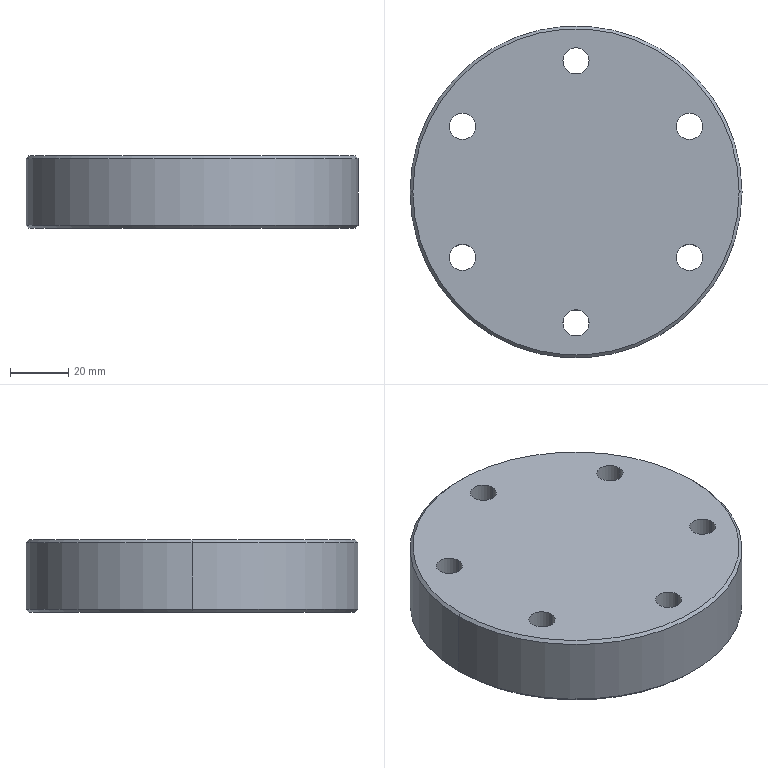Part | SolidWorks | features Chamfer 1, CirPattern 1, Extrusion 1, HoleWzd 1 | 1 solid | 38 faces | box 114 x 114 x 25 mm | volume 237134 mm3 | cylinder 26 | plane 8 | cone 4 | commonest cylinder face diameters 9 x12 15 x12 114 x2
STEP:
#1=CARTESIAN_POINT('',(46.471,22.5,12.));
#2=VERTEX_POINT('',#1);
#3=CARTESIAN_POINT('',(31.471,22.5,12.));
#4=VERTEX_POINT('',#3);
#5=CARTESIAN_POINT('',(38.971,22.5,12.));
#6=DIRECTION('',(0.,0.,-1.));
#7=DIRECTION('',(-1.,0.,0.));
#8=AXIS2_PLACEMENT_3D('',#5,#6,#7);
#9=CIRCLE('',#8,7.5);
#10=EDGE_CURVE('',#2,#4,#9,.T.);
#11=ORIENTED_EDGE('',*,*,#10,.F.);
#12=CARTESIAN_POINT('',(46.471,22.5,0.));
#13=VERTEX_POINT('',#12);
#14=CARTESIAN_POINT('',(46.471,22.5,0.));
#15=DIRECTION('',(0.,0.,-1.));
#16=VECTOR('',#15,1000.);
#17=LINE('',#14,#16);
#18=EDGE_CURVE('',#2,#13,#17,.T.);
#19=ORIENTED_EDGE('',*,*,#18,.T.);
#20=CARTESIAN_POINT('',(31.471,22.5,0.));
#21=VERTEX_POINT('',#20);
#22=CARTESIAN_POINT('',(38.971,22.5,0.));
#23=DIRECTION('',(0.,0.,-1.));
#24=DIRECTION('',(-1.,0.,0.));
#25=AXIS2_PLACEMENT_3D('',#22,#23,#24);
#26=CIRCLE('',#25,7.5);
#27=EDGE_CURVE('',#13,#21,#26,.T.);
#28=ORIENTED_EDGE('',*,*,#27,.T.);
#29=CARTESIAN_POINT('',(31.471,22.5,0.));
#30=DIRECTION('',(0.,0.,-1.));
#31=VECTOR('',#30,1000.);
#32=LINE('',#29,#31);
#33=EDGE_CURVE('',#4,#21,#32,.T.);
#34=ORIENTED_EDGE('',*,*,#33,.F.);
#35=EDGE_LOOP('',(#11,#19,#28,#34));
#36=FACE_OUTER_BOUND('',#35,.T.);
#37=CARTESIAN_POINT('',(38.971,22.5,0.));
#38=DIRECTION('',(0.,0.,-1.));
#39=DIRECTION('',(-1.,0.,0.));
#40=AXIS2_PLACEMENT_3D('',#37,#38,#39);
#41=CYLINDRICAL_SURFACE('',#40,7.5);
#42=ADVANCED_FACE('',(#36),#41,.F.);
#43=CARTESIAN_POINT('',(43.471,22.5,25.));
#44=VERTEX_POINT('',#43);
#45=CARTESIAN_POINT('',(34.471,22.5,25.));
#46=VERTEX_POINT('',#45);
#47=CARTESIAN_POINT('',(38.971,22.5,25.));
#48=DIRECTION('',(0.,0.,-1.));
#49=DIRECTION('',(-1.,0.,0.));
#50=AXIS2_PLACEMENT_3D('',#47,#48,#49);
#51=CIRCLE('',#50,4.5);
#52=EDGE_CURVE('',#44,#46,#51,.T.);
#53=ORIENTED_EDGE('',*,*,#52,.F.);
#54=CARTESIAN_POINT('',(43.471,22.5,12.));
#55=VERTEX_POINT('',#54);
#56=CARTESIAN_POINT('',(43.471,22.5,0.));
#57=DIRECTION('',(0.,0.,-1.));
#58=VECTOR('',#57,1000.);
#59=LINE('',#56,#58);
#60=EDGE_CURVE('',#44,#55,#59,.T.);
#61=ORIENTED_EDGE('',*,*,#60,.T.);
#62=CARTESIAN_POINT('',(34.471,22.5,12.));
#63=VERTEX_POINT('',#62);
#64=CARTESIAN_POINT('',(38.971,22.5,12.));
#65=DIRECTION('',(0.,0.,-1.));
#66=DIRECTION('',(-1.,0.,0.));
#67=AXIS2_PLACEMENT_3D('',#64,#65,#66);
#68=CIRCLE('',#67,4.5);
#69=EDGE_CURVE('',#55,#63,#68,.T.);
#70=ORIENTED_EDGE('',*,*,#69,.T.);
#71=CARTESIAN_POINT('',(34.471,22.5,0.));
#72=DIRECTION('',(0.,0.,-1.));
#73=VECTOR('',#72,1000.);
#74=LINE('',#71,#73);
#75=EDGE_CURVE('',#46,#63,#74,.T.);
#76=ORIENTED_EDGE('',*,*,#75,.F.);
#77=EDGE_LOOP('',(#53,#61,#70,#76));
#78=FACE_OUTER_BOUND('',#77,.T.);
#79=CARTESIAN_POINT('',(38.971,22.5,0.));
#80=DIRECTION('',(0.,0.,-1.));
#81=DIRECTION('',(-1.,0.,0.));
#82=AXIS2_PLACEMENT_3D('',#79,#80,#81);
#83=CYLINDRICAL_SURFACE('',#82,4.5);
#84=ADVANCED_FACE('',(#78),#83,.F.);
#85=CARTESIAN_POINT('',(46.471,-22.5,12.));
#86=VERTEX_POINT('',#85);
#87=CARTESIAN_POINT('',(31.471,-22.5,12.));
#88=VERTEX_POINT('',#87);
#89=CARTESIAN_POINT('',(38.971,-22.5,12.));
#90=DIRECTION('',(0.,0.,-1.));
#91=DIRECTION('',(-1.,0.,0.));
#92=AXIS2_PLACEMENT_3D('',#89,#90,#91);
#93=CIRCLE('',#92,7.5);
#94=EDGE_CURVE('',#86,#88,#93,.T.);
#95=ORIENTED_EDGE('',*,*,#94,.F.);
#96=CARTESIAN_POINT('',(46.471,-22.5,0.));
#97=VERTEX_POINT('',#96);
#98=CARTESIAN_POINT('',(46.471,-22.5,0.));
#99=DIRECTION('',(0.,0.,-1.));
#100=VECTOR('',#99,1000.);
#101=LINE('',#98,#100);
#102=EDGE_CURVE('',#86,#97,#101,.T.);
#103=ORIENTED_EDGE('',*,*,#102,.T.);
#104=CARTESIAN_POINT('',(31.471,-22.5,0.));
#105=VERTEX_POINT('',#104);
#106=CARTESIAN_POINT('',(38.971,-22.5,0.));
#107=DIRECTION('',(0.,0.,-1.));
#108=DIRECTION('',(-1.,0.,0.));
#109=AXIS2_PLACEMENT_3D('',#106,#107,#108);
#110=CIRCLE('',#109,7.5);
#111=EDGE_CURVE('',#97,#105,#110,.T.);
#112=ORIENTED_EDGE('',*,*,#111,.T.);
#113=CARTESIAN_POINT('',(31.471,-22.5,0.));
#114=DIRECTION('',(0.,0.,-1.));
#115=VECTOR('',#114,1000.);
#116=LINE('',#113,#115);
#117=EDGE_CURVE('',#88,#105,#116,.T.);
#118=ORIENTED_EDGE('',*,*,#117,.F.);
#119=EDGE_LOOP('',(#95,#103,#112,#118));
#120=FACE_OUTER_BOUND('',#119,.T.);
#121=CARTESIAN_POINT('',(38.971,-22.5,0.));
#122=DIRECTION('',(0.,0.,-1.));
#123=DIRECTION('',(-1.,0.,0.));
#124=AXIS2_PLACEMENT_3D('',#121,#122,#123);
#125=CYLINDRICAL_SURFACE('',#124,7.5);
#126=ADVANCED_FACE('',(#120),#125,.F.);
#127=CARTESIAN_POINT('',(43.471,-22.5,25.));
#128=VERTEX_POINT('',#127);
#129=CARTESIAN_POINT('',(34.471,-22.5,25.));
#130=VERTEX_POINT('',#129);
#131=CARTESIAN_POINT('',(38.971,-22.5,25.));
#132=DIRECTION('',(0.,0.,-1.));
#133=DIRECTION('',(-1.,0.,0.));
#134=AXIS2_PLACEMENT_3D('',#131,#132,#133);
#135=CIRCLE('',#134,4.5);
#136=EDGE_CURVE('',#128,#130,#135,.T.);
#137=ORIENTED_EDGE('',*,*,#136,.F.);
#138=CARTESIAN_POINT('',(43.471,-22.5,12.));
#139=VERTEX_POINT('',#138);
#140=CARTESIAN_POINT('',(43.471,-22.5,0.));
#141=DIRECTION('',(0.,0.,-1.));
#142=VECTOR('',#141,1000.);
#143=LINE('',#140,#142);
#144=EDGE_CURVE('',#128,#139,#143,.T.);
#145=ORIENTED_EDGE('',*,*,#144,.T.);
#146=CARTESIAN_POINT('',(34.471,-22.5,12.));
#147=VERTEX_POINT('',#146);
#148=CARTESIAN_POINT('',(38.971,-22.5,12.));
#149=DIRECTION('',(0.,0.,-1.));
#150=DIRECTION('',(-1.,0.,0.));
#151=AXIS2_PLACEMENT_3D('',#148,#149,#150);
#152=CIRCLE('',#151,4.5);
#153=EDGE_CURVE('',#139,#147,#152,.T.);
#154=ORIENTED_EDGE('',*,*,#153,.T.);
#155=CARTESIAN_POINT('',(34.471,-22.5,0.));
#156=DIRECTION('',(0.,0.,-1.));
#157=VECTOR('',#156,1000.);
#158=LINE('',#155,#157);
#159=EDGE_CURVE('',#130,#147,#158,.T.);
#160=ORIENTED_EDGE('',*,*,#159,.F.);
#161=EDGE_LOOP('',(#137,#145,#154,#160));
#162=FACE_OUTER_BOUND('',#161,.T.);
#163=CARTESIAN_POINT('',(38.971,-22.5,0.));
#164=DIRECTION('',(0.,0.,-1.));
#165=DIRECTION('',(-1.,0.,0.));
#166=AXIS2_PLACEMENT_3D('',#163,#164,#165);
#167=CYLINDRICAL_SURFACE('',#166,4.5);
#168=ADVANCED_FACE('',(#162),#167,.F.);
#169=CARTESIAN_POINT('',(7.5,-45.,12.));
#170=VERTEX_POINT('',#169);
#171=CARTESIAN_POINT('',(-7.5,-45.,12.));
#172=VERTEX_POINT('',#171);
#173=CARTESIAN_POINT('',(0.,-45.,12.));
#174=DIRECTION('',(0.,0.,-1.));
#175=DIRECTION('',(-1.,0.,0.));
#176=AXIS2_PLACEMENT_3D('',#173,#174,#175);
#177=CIRCLE('',#176,7.5);
#178=EDGE_CURVE('',#170,#172,#177,.T.);
#179=ORIENTED_EDGE('',*,*,#178,.F.);
#180=CARTESIAN_POINT('',(7.5,-45.,0.));
#181=VERTEX_POINT('',#180);
#182=CARTESIAN_POINT('',(7.5,-45.,0.));
#183=DIRECTION('',(0.,0.,-1.));
#184=VECTOR('',#183,1000.);
#185=LINE('',#182,#184);
#186=EDGE_CURVE('',#170,#181,#185,.T.);
#187=ORIENTED_EDGE('',*,*,#186,.T.);
#188=CARTESIAN_POINT('',(-7.5,-45.,0.));
#189=VERTEX_POINT('',#188);
#190=CARTESIAN_POINT('',(0.,-45.,0.));
#191=DIRECTION('',(0.,0.,-1.));
#192=DIRECTION('',(-1.,0.,0.));
#193=AXIS2_PLACEMENT_3D('',#190,#191,#192);
#194=CIRCLE('',#193,7.5);
#195=EDGE_CURVE('',#181,#189,#194,.T.);
#196=ORIENTED_EDGE('',*,*,#195,.T.);
#197=CARTESIAN_POINT('',(-7.5,-45.,0.));
#198=DIRECTION('',(0.,0.,-1.));
#199=VECTOR('',#198,1000.);
#200=LINE('',#197,#199);
#201=EDGE_CURVE('',#172,#189,#200,.T.);
#202=ORIENTED_EDGE('',*,*,#201,.F.);
#203=EDGE_LOOP('',(#179,#187,#196,#202));
#204=FACE_OUTER_BOUND('',#203,.T.);
#205=CARTESIAN_POINT('',(0.,-45.,0.));
#206=DIRECTION('',(0.,0.,-1.));
#207=DIRECTION('',(-1.,0.,0.));
#208=AXIS2_PLACEMENT_3D('',#205,#206,#207);
#209=CYLINDRICAL_SURFACE('',#208,7.5);
#210=ADVANCED_FACE('',(#204),#209,.F.);
#211=CARTESIAN_POINT('',(4.5,-45.,25.));
#212=VERTEX_POINT('',#211);
#213=CARTESIAN_POINT('',(-4.5,-45.,25.));
#214=VERTEX_POINT('',#213);
#215=CARTESIAN_POINT('',(0.,-45.,25.));
#216=DIRECTION('',(0.,0.,-1.));
#217=DIRECTION('',(-1.,0.,0.));
#218=AXIS2_PLACEMENT_3D('',#215,#216,#217);
#219=CIRCLE('',#218,4.5);
#220=EDGE_CURVE('',#212,#214,#219,.T.);
#221=ORIENTED_EDGE('',*,*,#220,.F.);
#222=CARTESIAN_POINT('',(4.5,-45.,12.));
#223=VERTEX_POINT('',#222);
#224=CARTESIAN_POINT('',(4.5,-45.,0.));
#225=DIRECTION('',(0.,0.,-1.));
#226=VECTOR('',#225,1000.);
#227=LINE('',#224,#226);
#228=EDGE_CURVE('',#212,#223,#227,.T.);
#229=ORIENTED_EDGE('',*,*,#228,.T.);
#230=CARTESIAN_POINT('',(-4.5,-45.,12.));
#231=VERTEX_POINT('',#230);
#232=CARTESIAN_POINT('',(0.,-45.,12.));
#233=DIRECTION('',(0.,0.,-1.));
#234=DIRECTION('',(-1.,0.,0.));
#235=AXIS2_PLACEMENT_3D('',#232,#233,#234);
#236=CIRCLE('',#235,4.5);
#237=EDGE_CURVE('',#223,#231,#236,.T.);
#238=ORIENTED_EDGE('',*,*,#237,.T.);
#239=CARTESIAN_POINT('',(-4.5,-45.,0.));
#240=DIRECTION('',(0.,0.,-1.));
#241=VECTOR('',#240,1000.);
#242=LINE('',#239,#241);
#243=EDGE_CURVE('',#214,#231,#242,.T.);
#244=ORIENTED_EDGE('',*,*,#243,.F.);
#245=EDGE_LOOP('',(#221,#229,#238,#244));
#246=FACE_OUTER_BOUND('',#245,.T.);
#247=CARTESIAN_POINT('',(0.,-45.,0.));
#248=DIRECTION('',(0.,0.,-1.));
#249=DIRECTION('',(-1.,0.,0.));
#250=AXIS2_PLACEMENT_3D('',#247,#248,#249);
#251=CYLINDRICAL_SURFACE('',#250,4.5);
#252=ADVANCED_FACE('',(#246),#251,.F.);
#253=CARTESIAN_POINT('',(-31.471,-22.5,12.));
#254=VERTEX_POINT('',#253);
#255=CARTESIAN_POINT('',(-46.471,-22.5,12.));
#256=VERTEX_POINT('',#255);
#257=CARTESIAN_POINT('',(-38.971,-22.5,12.));
#258=DIRECTION('',(0.,0.,-1.));
#259=DIRECTION('',(-1.,0.,0.));
#260=AXIS2_PLACEMENT_3D('',#257,#258,#259);
#261=CIRCLE('',#260,7.5);
#262=EDGE_CURVE('',#254,#256,#261,.T.);
#263=ORIENTED_EDGE('',*,*,#262,.F.);
#264=CARTESIAN_POINT('',(-31.471,-22.5,0.));
#265=VERTEX_POINT('',#264);
#266=CARTESIAN_POINT('',(-31.471,-22.5,0.));
#267=DIRECTION('',(0.,0.,-1.));
#268=VECTOR('',#267,1000.);
#269=LINE('',#266,#268);
#270=EDGE_CURVE('',#254,#265,#269,.T.);
#271=ORIENTED_EDGE('',*,*,#270,.T.);
#272=CARTESIAN_POINT('',(-46.471,-22.5,0.));
#273=VERTEX_POINT('',#272);
#274=CARTESIAN_POINT('',(-38.971,-22.5,0.));
#275=DIRECTION('',(0.,0.,-1.));
#276=DIRECTION('',(-1.,0.,0.));
#277=AXIS2_PLACEMENT_3D('',#274,#275,#276);
#278=CIRCLE('',#277,7.5);
#279=EDGE_CURVE('',#265,#273,#278,.T.);
#280=ORIENTED_EDGE('',*,*,#279,.T.);
#281=CARTESIAN_POINT('',(-46.471,-22.5,0.));
#282=DIRECTION('',(0.,0.,-1.));
#283=VECTOR('',#282,1000.);
#284=LINE('',#281,#283);
#285=EDGE_CURVE('',#256,#273,#284,.T.);
#286=ORIENTED_EDGE('',*,*,#285,.F.);
#287=EDGE_LOOP('',(#263,#271,#280,#286));
#288=FACE_OUTER_BOUND('',#287,.T.);
#289=CARTESIAN_POINT('',(-38.971,-22.5,0.));
#290=DIRECTION('',(0.,0.,-1.));
#291=DIRECTION('',(-1.,0.,0.));
#292=AXIS2_PLACEMENT_3D('',#289,#290,#291);
#293=CYLINDRICAL_SURFACE('',#292,7.5);
#294=ADVANCED_FACE('',(#288),#293,.F.);
#295=CARTESIAN_POINT('',(-34.471,-22.5,25.));
#296=VERTEX_POINT('',#295);
#297=CARTESIAN_POINT('',(-43.471,-22.5,25.));
#298=VERTEX_POINT('',#297);
#299=CARTESIAN_POINT('',(-38.971,-22.5,25.));
#300=DIRECTION('',(0.,0.,-1.));
#301=DIRECTION('',(-1.,0.,0.));
#302=AXIS2_PLACEMENT_3D('',#299,#300,#301);
#303=CIRCLE('',#302,4.5);
#304=EDGE_CURVE('',#296,#298,#303,.T.);
#305=ORIENTED_EDGE('',*,*,#304,.F.);
#306=CARTESIAN_POINT('',(-34.471,-22.5,12.));
#307=VERTEX_POINT('',#306);
#308=CARTESIAN_POINT('',(-34.471,-22.5,0.));
#309=DIRECTION('',(0.,0.,-1.));
#310=VECTOR('',#309,1000.);
#311=LINE('',#308,#310);
#312=EDGE_CURVE('',#296,#307,#311,.T.);
#313=ORIENTED_EDGE('',*,*,#312,.T.);
#314=CARTESIAN_POINT('',(-43.471,-22.5,12.));
#315=VERTEX_POINT('',#314);
#316=CARTESIAN_POINT('',(-38.971,-22.5,12.));
#317=DIRECTION('',(0.,0.,-1.));
#318=DIRECTION('',(-1.,0.,0.));
#319=AXIS2_PLACEMENT_3D('',#316,#317,#318);
#320=CIRCLE('',#319,4.5);
#321=EDGE_CURVE('',#307,#315,#320,.T.);
#322=ORIENTED_EDGE('',*,*,#321,.T.);
#323=CARTESIAN_POINT('',(-43.471,-22.5,0.));
#324=DIRECTION('',(0.,0.,-1.));
#325=VECTOR('',#324,1000.);
#326=LINE('',#323,#325);
#327=EDGE_CURVE('',#298,#315,#326,.T.);
#328=ORIENTED_EDGE('',*,*,#327,.F.);
#329=EDGE_LOOP('',(#305,#313,#322,#328));
#330=FACE_OUTER_BOUND('',#329,.T.);
#331=CARTESIAN_POINT('',(-38.971,-22.5,0.));
#332=DIRECTION('',(0.,0.,-1.));
#333=DIRECTION('',(-1.,0.,0.));
#334=AXIS2_PLACEMENT_3D('',#331,#332,#333);
#335=CYLINDRICAL_SURFACE('',#334,4.5);
#336=ADVANCED_FACE('',(#330),#335,.F.);
#337=CARTESIAN_POINT('',(-31.471,22.5,12.));
#338=VERTEX_POINT('',#337);
#339=CARTESIAN_POINT('',(-46.471,22.5,12.));
#340=VERTEX_POINT('',#339);
#341=CARTESIAN_POINT('',(-38.971,22.5,12.));
#342=DIRECTION('',(0.,0.,-1.));
#343=DIRECTION('',(-1.,0.,0.));
#344=AXIS2_PLACEMENT_3D('',#341,#342,#343);
#345=CIRCLE('',#344,7.5);
#346=EDGE_CURVE('',#338,#340,#345,.T.);
#347=ORIENTED_EDGE('',*,*,#346,.F.);
#348=CARTESIAN_POINT('',(-31.471,22.5,0.));
#349=VERTEX_POINT('',#348);
#350=CARTESIAN_POINT('',(-31.471,22.5,0.));
#351=DIRECTION('',(0.,0.,-1.));
#352=VECTOR('',#351,1000.);
#353=LINE('',#350,#352);
#354=EDGE_CURVE('',#338,#349,#353,.T.);
#355=ORIENTED_EDGE('',*,*,#354,.T.);
#356=CARTESIAN_POINT('',(-46.471,22.5,0.));
#357=VERTEX_POINT('',#356);
#358=CARTESIAN_POINT('',(-38.971,22.5,0.));
#359=DIRECTION('',(0.,0.,-1.));
#360=DIRECTION('',(-1.,0.,0.));
#361=AXIS2_PLACEMENT_3D('',#358,#359,#360);
#362=CIRCLE('',#361,7.5);
#363=EDGE_CURVE('',#349,#357,#362,.T.);
#364=ORIENTED_EDGE('',*,*,#363,.T.);
#365=CARTESIAN_POINT('',(-46.471,22.5,0.));
#366=DIRECTION('',(0.,0.,-1.));
#367=VECTOR('',#366,1000.);
#368=LINE('',#365,#367);
#369=EDGE_CURVE('',#340,#357,#368,.T.);
#370=ORIENTED_EDGE('',*,*,#369,.F.);
#371=EDGE_LOOP('',(#347,#355,#364,#370));
#372=FACE_OUTER_BOUND('',#371,.T.);
#373=CARTESIAN_POINT('',(-38.971,22.5,0.));
#374=DIRECTION('',(0.,0.,-1.));
#375=DIRECTION('',(-1.,0.,0.));
#376=AXIS2_PLACEMENT_3D('',#373,#374,#375);
#377=CYLINDRICAL_SURFACE('',#376,7.5);
#378=ADVANCED_FACE('',(#372),#377,.F.);
#379=CARTESIAN_POINT('',(-34.471,22.5,25.));
#380=VERTEX_POINT('',#379);
#381=CARTESIAN_POINT('',(-43.471,22.5,25.));
#382=VERTEX_POINT('',#381);
#383=CARTESIAN_POINT('',(-38.971,22.5,25.));
#384=DIRECTION('',(0.,0.,-1.));
#385=DIRECTION('',(-1.,0.,0.));
#386=AXIS2_PLACEMENT_3D('',#383,#384,#385);
#387=CIRCLE('',#386,4.5);
#388=EDGE_CURVE('',#380,#382,#387,.T.);
#389=ORIENTED_EDGE('',*,*,#388,.F.);
#390=CARTESIAN_POINT('',(-34.471,22.5,12.));
#391=VERTEX_POINT('',#390);
#392=CARTESIAN_POINT('',(-34.471,22.5,0.));
#393=DIRECTION('',(0.,0.,-1.));
#394=VECTOR('',#393,1000.);
#395=LINE('',#392,#394);
#396=EDGE_CURVE('',#380,#391,#395,.T.);
#397=ORIENTED_EDGE('',*,*,#396,.T.);
#398=CARTESIAN_POINT('',(-43.471,22.5,12.));
#399=VERTEX_POINT('',#398);
#400=CARTESIAN_POINT('',(-38.971,22.5,12.));
#401=DIRECTION('',(0.,0.,-1.));
#402=DIRECTION('',(-1.,0.,0.));
#403=AXIS2_PLACEMENT_3D('',#400,#401,#402);
#404=CIRCLE('',#403,4.5);
#405=EDGE_CURVE('',#391,#399,#404,.T.);
#406=ORIENTED_EDGE('',*,*,#405,.T.);
#407=CARTESIAN_POINT('',(-43.471,22.5,0.));
#408=DIRECTION('',(0.,0.,-1.));
#409=VECTOR('',#408,1000.);
#410=LINE('',#407,#409);
#411=EDGE_CURVE('',#382,#399,#410,.T.);
#412=ORIENTED_EDGE('',*,*,#411,.F.);
#413=EDGE_LOOP('',(#389,#397,#406,#412));
#414=FACE_OUTER_BOUND('',#413,.T.);
#415=CARTESIAN_POINT('',(-38.971,22.5,0.));
#416=DIRECTION('',(0.,0.,-1.));
#417=DIRECTION('',(-1.,0.,0.));
#418=AXIS2_PLACEMENT_3D('',#415,#416,#417);
#419=CYLINDRICAL_SURFACE('',#418,4.5);
#420=ADVANCED_FACE('',(#414),#419,.F.);
#421=CARTESIAN_POINT('',(7.5,45.,12.));
#422=VERTEX_POINT('',#421);
#423=CARTESIAN_POINT('',(-7.5,45.,12.));
#424=VERTEX_POINT('',#423);
#425=CARTESIAN_POINT('',(0.,45.,12.));
#426=DIRECTION('',(0.,0.,-1.));
#427=DIRECTION('',(-1.,0.,0.));
#428=AXIS2_PLACEMENT_3D('',#425,#426,#427);
#429=CIRCLE('',#428,7.5);
#430=EDGE_CURVE('',#422,#424,#429,.T.);
#431=ORIENTED_EDGE('',*,*,#430,.F.);
#432=CARTESIAN_POINT('',(7.5,45.,0.));
#433=VERTEX_POINT('',#432);
#434=CARTESIAN_POINT('',(7.5,45.,0.));
#435=DIRECTION('',(0.,0.,-1.));
#436=VECTOR('',#435,1000.);
#437=LINE('',#434,#436);
#438=EDGE_CURVE('',#422,#433,#437,.T.);
#439=ORIENTED_EDGE('',*,*,#438,.T.);
#440=CARTESIAN_POINT('',(-7.5,45.,0.));
#441=VERTEX_POINT('',#440);
#442=CARTESIAN_POINT('',(0.,45.,0.));
#443=DIRECTION('',(0.,0.,-1.));
#444=DIRECTION('',(-1.,0.,0.));
#445=AXIS2_PLACEMENT_3D('',#442,#443,#444);
#446=CIRCLE('',#445,7.5);
#447=EDGE_CURVE('',#433,#441,#446,.T.);
#448=ORIENTED_EDGE('',*,*,#447,.T.);
#449=CARTESIAN_POINT('',(-7.5,45.,0.));
#450=DIRECTION('',(0.,0.,-1.));
#451=VECTOR('',#450,1000.);
#452=LINE('',#449,#451);
#453=EDGE_CURVE('',#424,#441,#452,.T.);
#454=ORIENTED_EDGE('',*,*,#453,.F.);
#455=EDGE_LOOP('',(#431,#439,#448,#454));
#456=FACE_OUTER_BOUND('',#455,.T.);
#457=CARTESIAN_POINT('',(0.,45.,0.));
#458=DIRECTION('',(0.,0.,-1.));
#459=DIRECTION('',(-1.,0.,0.));
#460=AXIS2_PLACEMENT_3D('',#457,#458,#459);
#461=CYLINDRICAL_SURFACE('',#460,7.5);
#462=ADVANCED_FACE('',(#456),#461,.F.);
#463=CARTESIAN_POINT('',(4.5,45.,25.));
#464=VERTEX_POINT('',#463);
#465=CARTESIAN_POINT('',(-4.5,45.,25.));
#466=VERTEX_POINT('',#465);
#467=CARTESIAN_POINT('',(0.,45.,25.));
#468=DIRECTION('',(0.,0.,-1.));
#469=DIRECTION('',(-1.,0.,0.));
#470=AXIS2_PLACEMENT_3D('',#467,#468,#469);
#471=CIRCLE('',#470,4.5);
#472=EDGE_CURVE('',#464,#466,#471,.T.);
#473=ORIENTED_EDGE('',*,*,#472,.F.);
#474=CARTESIAN_POINT('',(4.5,45.,12.));
#475=VERTEX_POINT('',#474);
#476=CARTESIAN_POINT('',(4.5,45.,0.));
#477=DIRECTION('',(0.,0.,-1.));
#478=VECTOR('',#477,1000.);
#479=LINE('',#476,#478);
#480=EDGE_CURVE('',#464,#475,#479,.T.);
#481=ORIENTED_EDGE('',*,*,#480,.T.);
#482=CARTESIAN_POINT('',(-4.5,45.,12.));
#483=VERTEX_POINT('',#482);
#484=CARTESIAN_POINT('',(0.,45.,12.));
#485=DIRECTION('',(0.,0.,-1.));
#486=DIRECTION('',(-1.,0.,0.));
#487=AXIS2_PLACEMENT_3D('',#484,#485,#486);
#488=CIRCLE('',#487,4.5);
#489=EDGE_CURVE('',#475,#483,#488,.T.);
#490=ORIENTED_EDGE('',*,*,#489,.T.);
#491=CARTESIAN_POINT('',(-4.5,45.,0.));
#492=DIRECTION('',(0.,0.,-1.));
#493=VECTOR('',#492,1000.);
#494=LINE('',#491,#493);
#495=EDGE_CURVE('',#466,#483,#494,.T.);
#496=ORIENTED_EDGE('',*,*,#495,.F.);
#497=EDGE_LOOP('',(#473,#481,#490,#496));
#498=FACE_OUTER_BOUND('',#497,.T.);
#499=CARTESIAN_POINT('',(0.,45.,0.));
#500=DIRECTION('',(0.,0.,-1.));
#501=DIRECTION('',(-1.,0.,0.));
#502=AXIS2_PLACEMENT_3D('',#499,#500,#501);
#503=CYLINDRICAL_SURFACE('',#502,4.5);
#504=ADVANCED_FACE('',(#498),#503,.F.);
#505=CARTESIAN_POINT('',(-56.,0.,0.));
#506=VERTEX_POINT('',#505);
#507=CARTESIAN_POINT('',(56.,0.,0.));
#508=VERTEX_POINT('',#507);
#509=CARTESIAN_POINT('',(0.,0.,0.));
#510=DIRECTION('',(0.,0.,-1.));
#511=DIRECTION('',(1.,0.,0.));
#512=AXIS2_PLACEMENT_3D('',#509,#510,#511);
#513=CIRCLE('',#512,56.);
#514=EDGE_CURVE('',#506,#508,#513,.T.);
#515=ORIENTED_EDGE('',*,*,#514,.F.);
#516=CARTESIAN_POINT('',(-57.,0.,1.));
#517=VERTEX_POINT('',#516);
#518=CARTESIAN_POINT('',(-57.,0.,1.));
#519=DIRECTION('',(-0.7071,0.,0.7071));
#520=VECTOR('',#519,1000.);
#521=LINE('',#518,#520);
#522=EDGE_CURVE('',#506,#517,#521,.T.);
#523=ORIENTED_EDGE('',*,*,#522,.T.);
#524=CARTESIAN_POINT('',(57.,0.,1.));
#525=VERTEX_POINT('',#524);
#526=CARTESIAN_POINT('',(0.,0.,1.));
#527=DIRECTION('',(0.,0.,1.));
#528=DIRECTION('',(1.,0.,0.));
#529=AXIS2_PLACEMENT_3D('',#526,#527,#528);
#530=CIRCLE('',#529,57.);
#531=EDGE_CURVE('',#525,#517,#530,.T.);
#532=ORIENTED_EDGE('',*,*,#531,.F.);
#533=CARTESIAN_POINT('',(57.,0.,1.));
#534=DIRECTION('',(0.7071,0.,0.7071));
#535=VECTOR('',#534,1000.);
#536=LINE('',#533,#535);
#537=EDGE_CURVE('',#508,#525,#536,.T.);
#538=ORIENTED_EDGE('',*,*,#537,.F.);
#539=EDGE_LOOP('',(#515,#523,#532,#538));
#540=FACE_OUTER_BOUND('',#539,.T.);
#541=CARTESIAN_POINT('',(0.,0.,1.));
#542=DIRECTION('',(0.,0.,1.));
#543=DIRECTION('',(1.,0.,0.));
#544=AXIS2_PLACEMENT_3D('',#541,#542,#543);
#545=CONICAL_SURFACE('',#544,57.,0.7854);
#546=ADVANCED_FACE('',(#540),#545,.T.);
#547=CARTESIAN_POINT('',(56.,0.,25.));
#548=VERTEX_POINT('',#547);
#549=CARTESIAN_POINT('',(-56.,0.,25.));
#550=VERTEX_POINT('',#549);
#551=CARTESIAN_POINT('',(0.,0.,25.));
#552=DIRECTION('',(0.,0.,1.));
#553=DIRECTION('',(1.,0.,0.));
#554=AXIS2_PLACEMENT_3D('',#551,#552,#553);
#555=CIRCLE('',#554,56.);
#556=EDGE_CURVE('',#548,#550,#555,.T.);
#557=ORIENTED_EDGE('',*,*,#556,.F.);
#558=CARTESIAN_POINT('',(57.,0.,24.));
#559=VERTEX_POINT('',#558);
#560=CARTESIAN_POINT('',(56.,0.,25.));
#561=DIRECTION('',(0.7071,0.,-0.7071));
#562=VECTOR('',#561,1000.);
#563=LINE('',#560,#562);
#564=EDGE_CURVE('',#548,#559,#563,.T.);
#565=ORIENTED_EDGE('',*,*,#564,.T.);
#566=CARTESIAN_POINT('',(-57.,0.,24.));
#567=VERTEX_POINT('',#566);
#568=CARTESIAN_POINT('',(0.,0.,24.));
#569=DIRECTION('',(0.,0.,-1.));
#570=DIRECTION('',(1.,0.,0.));
#571=AXIS2_PLACEMENT_3D('',#568,#569,#570);
#572=CIRCLE('',#571,57.);
#573=EDGE_CURVE('',#567,#559,#572,.T.);
#574=ORIENTED_EDGE('',*,*,#573,.F.);
#575=CARTESIAN_POINT('',(-56.,0.,25.));
#576=DIRECTION('',(-0.7071,0.,-0.7071));
#577=VECTOR('',#576,1000.);
#578=LINE('',#575,#577);
#579=EDGE_CURVE('',#550,#567,#578,.T.);
#580=ORIENTED_EDGE('',*,*,#579,.F.);
#581=EDGE_LOOP('',(#557,#565,#574,#580));
#582=FACE_OUTER_BOUND('',#581,.T.);
#583=CARTESIAN_POINT('',(0.,0.,25.));
#584=DIRECTION('',(0.,0.,-1.));
#585=DIRECTION('',(-1.,0.,0.));
#586=AXIS2_PLACEMENT_3D('',#583,#584,#585);
#587=CONICAL_SURFACE('',#586,56.,0.7854);
#588=ADVANCED_FACE('',(#582),#587,.T.);
#589=ORIENTED_EDGE('',*,*,#573,.T.);
#590=CARTESIAN_POINT('',(57.,0.,25.));
#591=DIRECTION('',(0.,0.,-1.));
#592=VECTOR('',#591,1000.);
#593=LINE('',#590,#592);
#594=EDGE_CURVE('',#559,#525,#593,.T.);
#595=ORIENTED_EDGE('',*,*,#594,.T.);
#596=ORIENTED_EDGE('',*,*,#531,.T.);
#597=CARTESIAN_POINT('',(-57.,0.,25.));
#598=DIRECTION('',(0.,0.,-1.));
#599=VECTOR('',#598,1000.);
#600=LINE('',#597,#599);
#601=EDGE_CURVE('',#567,#517,#600,.T.);
#602=ORIENTED_EDGE('',*,*,#601,.F.);
#603=EDGE_LOOP('',(#589,#595,#596,#602));
#604=FACE_OUTER_BOUND('',#603,.T.);
#605=CARTESIAN_POINT('',(0.,0.,25.));
#606=DIRECTION('',(0.,0.,-1.));
#607=DIRECTION('',(-1.,0.,0.));
#608=AXIS2_PLACEMENT_3D('',#605,#606,#607);
#609=CYLINDRICAL_SURFACE('',#608,57.);
#610=ADVANCED_FACE('',(#604),#609,.T.);
#611=CARTESIAN_POINT('',(38.971,-22.5,0.));
#612=DIRECTION('',(0.,0.,-1.));
#613=DIRECTION('',(-1.,0.,0.));
#614=AXIS2_PLACEMENT_3D('',#611,#612,#613);
#615=CIRCLE('',#614,7.5);
#616=EDGE_CURVE('',#105,#97,#615,.T.);
#617=ORIENTED_EDGE('',*,*,#616,.F.);
#618=ORIENTED_EDGE('',*,*,#111,.F.);
#619=EDGE_LOOP('',(#617,#618));
#620=FACE_BOUND('',#619,.T.);
#621=CARTESIAN_POINT('',(0.,-45.,0.));
#622=DIRECTION('',(0.,0.,-1.));
#623=DIRECTION('',(-1.,0.,0.));
#624=AXIS2_PLACEMENT_3D('',#621,#622,#623);
#625=CIRCLE('',#624,7.5);
#626=EDGE_CURVE('',#189,#181,#625,.T.);
#627=ORIENTED_EDGE('',*,*,#626,.F.);
#628=ORIENTED_EDGE('',*,*,#195,.F.);
#629=EDGE_LOOP('',(#627,#628));
#630=FACE_BOUND('',#629,.T.);
#631=CARTESIAN_POINT('',(-38.971,-22.5,0.));
#632=DIRECTION('',(0.,0.,-1.));
#633=DIRECTION('',(-1.,0.,0.));
#634=AXIS2_PLACEMENT_3D('',#631,#632,#633);
#635=CIRCLE('',#634,7.5);
#636=EDGE_CURVE('',#273,#265,#635,.T.);
#637=ORIENTED_EDGE('',*,*,#636,.F.);
#638=ORIENTED_EDGE('',*,*,#279,.F.);
#639=EDGE_LOOP('',(#637,#638));
#640=FACE_BOUND('',#639,.T.);
#641=CARTESIAN_POINT('',(-38.971,22.5,0.));
#642=DIRECTION('',(0.,0.,-1.));
#643=DIRECTION('',(-1.,0.,0.));
#644=AXIS2_PLACEMENT_3D('',#641,#642,#643);
#645=CIRCLE('',#644,7.5);
#646=EDGE_CURVE('',#357,#349,#645,.T.);
#647=ORIENTED_EDGE('',*,*,#646,.F.);
#648=ORIENTED_EDGE('',*,*,#363,.F.);
#649=EDGE_LOOP('',(#647,#648));
#650=FACE_BOUND('',#649,.T.);
#651=CARTESIAN_POINT('',(0.,45.,0.));
#652=DIRECTION('',(0.,0.,-1.));
#653=DIRECTION('',(-1.,0.,0.));
#654=AXIS2_PLACEMENT_3D('',#651,#652,#653);
#655=CIRCLE('',#654,7.5);
#656=EDGE_CURVE('',#441,#433,#655,.T.);
#657=ORIENTED_EDGE('',*,*,#656,.F.);
#658=ORIENTED_EDGE('',*,*,#447,.F.);
#659=EDGE_LOOP('',(#657,#658));
#660=FACE_BOUND('',#659,.T.);
#661=CARTESIAN_POINT('',(0.,0.,0.));
#662=DIRECTION('',(0.,0.,-1.));
#663=DIRECTION('',(1.,0.,0.));
#664=AXIS2_PLACEMENT_3D('',#661,#662,#663);
#665=CIRCLE('',#664,56.);
#666=EDGE_CURVE('',#508,#506,#665,.T.);
#667=ORIENTED_EDGE('',*,*,#666,.T.);
#668=ORIENTED_EDGE('',*,*,#514,.T.);
#669=EDGE_LOOP('',(#667,#668));
#670=FACE_OUTER_BOUND('',#669,.T.);
#671=CARTESIAN_POINT('',(38.971,22.5,0.));
#672=DIRECTION('',(0.,0.,-1.));
#673=DIRECTION('',(-1.,0.,0.));
#674=AXIS2_PLACEMENT_3D('',#671,#672,#673);
#675=CIRCLE('',#674,7.5);
#676=EDGE_CURVE('',#21,#13,#675,.T.);
#677=ORIENTED_EDGE('',*,*,#676,.F.);
#678=ORIENTED_EDGE('',*,*,#27,.F.);
#679=EDGE_LOOP('',(#677,#678));
#680=FACE_BOUND('',#679,.T.);
#681=CARTESIAN_POINT('',(0.,0.,0.));
#682=DIRECTION('',(0.,0.,1.));
#683=DIRECTION('',(1.,0.,0.));
#684=AXIS2_PLACEMENT_3D('',#681,#682,#683);
#685=PLANE('',#684);
#686=ADVANCED_FACE('',(#620,#630,#640,#650,#660,#670,#680),#685,.F.);
#687=ORIENTED_EDGE('',*,*,#594,.F.);
#688=CARTESIAN_POINT('',(0.,0.,24.));
#689=DIRECTION('',(0.,0.,-1.));
#690=DIRECTION('',(1.,0.,0.));
#691=AXIS2_PLACEMENT_3D('',#688,#689,#690);
#692=CIRCLE('',#691,57.);
#693=EDGE_CURVE('',#559,#567,#692,.T.);
#694=ORIENTED_EDGE('',*,*,#693,.T.);
#695=ORIENTED_EDGE('',*,*,#601,.T.);
#696=CARTESIAN_POINT('',(0.,0.,1.));
#697=DIRECTION('',(0.,0.,1.));
#698=DIRECTION('',(1.,0.,0.));
#699=AXIS2_PLACEMENT_3D('',#696,#697,#698);
#700=CIRCLE('',#699,57.);
#701=EDGE_CURVE('',#517,#525,#700,.T.);
#702=ORIENTED_EDGE('',*,*,#701,.T.);
#703=EDGE_LOOP('',(#687,#694,#695,#702));
#704=FACE_OUTER_BOUND('',#703,.T.);
#705=CARTESIAN_POINT('',(0.,0.,25.));
#706=DIRECTION('',(0.,0.,-1.));
#707=DIRECTION('',(-1.,0.,0.));
#708=AXIS2_PLACEMENT_3D('',#705,#706,#707);
#709=CYLINDRICAL_SURFACE('',#708,57.);
#710=ADVANCED_FACE('',(#704),#709,.T.);
#711=CARTESIAN_POINT('',(38.971,22.5,25.));
#712=DIRECTION('',(0.,0.,-1.));
#713=DIRECTION('',(-1.,0.,0.));
#714=AXIS2_PLACEMENT_3D('',#711,#712,#713);
#715=CIRCLE('',#714,4.5);
#716=EDGE_CURVE('',#46,#44,#715,.T.);
#717=ORIENTED_EDGE('',*,*,#716,.T.);
#718=ORIENTED_EDGE('',*,*,#52,.T.);
#719=EDGE_LOOP('',(#717,#718));
#720=FACE_BOUND('',#719,.T.);
#721=CARTESIAN_POINT('',(38.971,-22.5,25.));
#722=DIRECTION('',(0.,0.,-1.));
#723=DIRECTION('',(-1.,0.,0.));
#724=AXIS2_PLACEMENT_3D('',#721,#722,#723);
#725=CIRCLE('',#724,4.5);
#726=EDGE_CURVE('',#130,#128,#725,.T.);
#727=ORIENTED_EDGE('',*,*,#726,.T.);
#728=ORIENTED_EDGE('',*,*,#136,.T.);
#729=EDGE_LOOP('',(#727,#728));
#730=FACE_BOUND('',#729,.T.);
#731=CARTESIAN_POINT('',(0.,-45.,25.));
#732=DIRECTION('',(0.,0.,-1.));
#733=DIRECTION('',(-1.,0.,0.));
#734=AXIS2_PLACEMENT_3D('',#731,#732,#733);
#735=CIRCLE('',#734,4.5);
#736=EDGE_CURVE('',#214,#212,#735,.T.);
#737=ORIENTED_EDGE('',*,*,#736,.T.);
#738=ORIENTED_EDGE('',*,*,#220,.T.);
#739=EDGE_LOOP('',(#737,#738));
#740=FACE_BOUND('',#739,.T.);
#741=CARTESIAN_POINT('',(-38.971,-22.5,25.));
#742=DIRECTION('',(0.,0.,-1.));
#743=DIRECTION('',(-1.,0.,0.));
#744=AXIS2_PLACEMENT_3D('',#741,#742,#743);
#745=CIRCLE('',#744,4.5);
#746=EDGE_CURVE('',#298,#296,#745,.T.);
#747=ORIENTED_EDGE('',*,*,#746,.T.);
#748=ORIENTED_EDGE('',*,*,#304,.T.);
#749=EDGE_LOOP('',(#747,#748));
#750=FACE_BOUND('',#749,.T.);
#751=CARTESIAN_POINT('',(-38.971,22.5,25.));
#752=DIRECTION('',(0.,0.,-1.));
#753=DIRECTION('',(-1.,0.,0.));
#754=AXIS2_PLACEMENT_3D('',#751,#752,#753);
#755=CIRCLE('',#754,4.5);
#756=EDGE_CURVE('',#382,#380,#755,.T.);
#757=ORIENTED_EDGE('',*,*,#756,.T.);
#758=ORIENTED_EDGE('',*,*,#388,.T.);
#759=EDGE_LOOP('',(#757,#758));
#760=FACE_BOUND('',#759,.T.);
#761=CARTESIAN_POINT('',(0.,45.,25.));
#762=DIRECTION('',(0.,0.,-1.));
#763=DIRECTION('',(-1.,0.,0.));
#764=AXIS2_PLACEMENT_3D('',#761,#762,#763);
#765=CIRCLE('',#764,4.5);
#766=EDGE_CURVE('',#466,#464,#765,.T.);
#767=ORIENTED_EDGE('',*,*,#766,.T.);
#768=ORIENTED_EDGE('',*,*,#472,.T.);
#769=EDGE_LOOP('',(#767,#768));
#770=FACE_BOUND('',#769,.T.);
#771=CARTESIAN_POINT('',(0.,0.,25.));
#772=DIRECTION('',(0.,0.,1.));
#773=DIRECTION('',(1.,0.,0.));
#774=AXIS2_PLACEMENT_3D('',#771,#772,#773);
#775=CIRCLE('',#774,56.);
#776=EDGE_CURVE('',#550,#548,#775,.T.);
#777=ORIENTED_EDGE('',*,*,#776,.T.);
#778=ORIENTED_EDGE('',*,*,#556,.T.);
#779=EDGE_LOOP('',(#777,#778));
#780=FACE_OUTER_BOUND('',#779,.T.);
#781=CARTESIAN_POINT('',(0.,0.,25.));
#782=DIRECTION('',(0.,0.,1.));
#783=DIRECTION('',(1.,0.,0.));
#784=AXIS2_PLACEMENT_3D('',#781,#782,#783);
#785=PLANE('',#784);
#786=ADVANCED_FACE('',(#720,#730,#740,#750,#760,#770,#780),#785,.T.);
#787=ORIENTED_EDGE('',*,*,#564,.F.);
#788=ORIENTED_EDGE('',*,*,#776,.F.);
#789=ORIENTED_EDGE('',*,*,#579,.T.);
#790=ORIENTED_EDGE('',*,*,#693,.F.);
#791=EDGE_LOOP('',(#787,#788,#789,#790));
#792=FACE_OUTER_BOUND('',#791,.T.);
#793=CARTESIAN_POINT('',(0.,0.,25.));
#794=DIRECTION('',(0.,0.,-1.));
#795=DIRECTION('',(-1.,0.,0.));
#796=AXIS2_PLACEMENT_3D('',#793,#794,#795);
#797=CONICAL_SURFACE('',#796,56.,0.7854);
#798=ADVANCED_FACE('',(#792),#797,.T.);
#799=ORIENTED_EDGE('',*,*,#522,.F.);
#800=ORIENTED_EDGE('',*,*,#666,.F.);
#801=ORIENTED_EDGE('',*,*,#537,.T.);
#802=ORIENTED_EDGE('',*,*,#701,.F.);
#803=EDGE_LOOP('',(#799,#800,#801,#802));
#804=FACE_OUTER_BOUND('',#803,.T.);
#805=CARTESIAN_POINT('',(0.,0.,1.));
#806=DIRECTION('',(0.,0.,1.));
#807=DIRECTION('',(1.,0.,0.));
#808=AXIS2_PLACEMENT_3D('',#805,#806,#807);
#809=CONICAL_SURFACE('',#808,57.,0.7854);
#810=ADVANCED_FACE('',(#804),#809,.T.);
#811=ORIENTED_EDGE('',*,*,#480,.F.);
#812=ORIENTED_EDGE('',*,*,#766,.F.);
#813=ORIENTED_EDGE('',*,*,#495,.T.);
#814=CARTESIAN_POINT('',(0.,45.,12.));
#815=DIRECTION('',(0.,0.,-1.));
#816=DIRECTION('',(-1.,0.,0.));
#817=AXIS2_PLACEMENT_3D('',#814,#815,#816);
#818=CIRCLE('',#817,4.5);
#819=EDGE_CURVE('',#483,#475,#818,.T.);
#820=ORIENTED_EDGE('',*,*,#819,.T.);
#821=EDGE_LOOP('',(#811,#812,#813,#820));
#822=FACE_OUTER_BOUND('',#821,.T.);
#823=CARTESIAN_POINT('',(0.,45.,0.));
#824=DIRECTION('',(0.,0.,-1.));
#825=DIRECTION('',(-1.,0.,0.));
#826=AXIS2_PLACEMENT_3D('',#823,#824,#825);
#827=CYLINDRICAL_SURFACE('',#826,4.5);
#828=ADVANCED_FACE('',(#822),#827,.F.);
#829=ORIENTED_EDGE('',*,*,#819,.F.);
#830=ORIENTED_EDGE('',*,*,#489,.F.);
#831=EDGE_LOOP('',(#829,#830));
#832=FACE_BOUND('',#831,.T.);
#833=CARTESIAN_POINT('',(0.,45.,12.));
#834=DIRECTION('',(0.,0.,-1.));
#835=DIRECTION('',(-1.,0.,0.));
#836=AXIS2_PLACEMENT_3D('',#833,#834,#835);
#837=CIRCLE('',#836,7.5);
#838=EDGE_CURVE('',#424,#422,#837,.T.);
#839=ORIENTED_EDGE('',*,*,#838,.T.);
#840=ORIENTED_EDGE('',*,*,#430,.T.);
#841=EDGE_LOOP('',(#839,#840));
#842=FACE_OUTER_BOUND('',#841,.T.);
#843=CARTESIAN_POINT('',(4.5,45.,12.));
#844=DIRECTION('',(0.,0.,1.));
#845=DIRECTION('',(1.,0.,0.));
#846=AXIS2_PLACEMENT_3D('',#843,#844,#845);
#847=PLANE('',#846);
#848=ADVANCED_FACE('',(#832,#842),#847,.F.);
#849=ORIENTED_EDGE('',*,*,#438,.F.);
#850=ORIENTED_EDGE('',*,*,#838,.F.);
#851=ORIENTED_EDGE('',*,*,#453,.T.);
#852=ORIENTED_EDGE('',*,*,#656,.T.);
#853=EDGE_LOOP('',(#849,#850,#851,#852));
#854=FACE_OUTER_BOUND('',#853,.T.);
#855=CARTESIAN_POINT('',(0.,45.,0.));
#856=DIRECTION('',(0.,0.,-1.));
#857=DIRECTION('',(-1.,0.,0.));
#858=AXIS2_PLACEMENT_3D('',#855,#856,#857);
#859=CYLINDRICAL_SURFACE('',#858,7.5);
#860=ADVANCED_FACE('',(#854),#859,.F.);
#861=ORIENTED_EDGE('',*,*,#396,.F.);
#862=ORIENTED_EDGE('',*,*,#756,.F.);
#863=ORIENTED_EDGE('',*,*,#411,.T.);
#864=CARTESIAN_POINT('',(-38.971,22.5,12.));
#865=DIRECTION('',(0.,0.,-1.));
#866=DIRECTION('',(-1.,0.,0.));
#867=AXIS2_PLACEMENT_3D('',#864,#865,#866);
#868=CIRCLE('',#867,4.5);
#869=EDGE_CURVE('',#399,#391,#868,.T.);
#870=ORIENTED_EDGE('',*,*,#869,.T.);
#871=EDGE_LOOP('',(#861,#862,#863,#870));
#872=FACE_OUTER_BOUND('',#871,.T.);
#873=CARTESIAN_POINT('',(-38.971,22.5,0.));
#874=DIRECTION('',(0.,0.,-1.));
#875=DIRECTION('',(-1.,0.,0.));
#876=AXIS2_PLACEMENT_3D('',#873,#874,#875);
#877=CYLINDRICAL_SURFACE('',#876,4.5);
#878=ADVANCED_FACE('',(#872),#877,.F.);
#879=ORIENTED_EDGE('',*,*,#869,.F.);
#880=ORIENTED_EDGE('',*,*,#405,.F.);
#881=EDGE_LOOP('',(#879,#880));
#882=FACE_BOUND('',#881,.T.);
#883=CARTESIAN_POINT('',(-38.971,22.5,12.));
#884=DIRECTION('',(0.,0.,-1.));
#885=DIRECTION('',(-1.,0.,0.));
#886=AXIS2_PLACEMENT_3D('',#883,#884,#885);
#887=CIRCLE('',#886,7.5);
#888=EDGE_CURVE('',#340,#338,#887,.T.);
#889=ORIENTED_EDGE('',*,*,#888,.T.);
#890=ORIENTED_EDGE('',*,*,#346,.T.);
#891=EDGE_LOOP('',(#889,#890));
#892=FACE_OUTER_BOUND('',#891,.T.);
#893=CARTESIAN_POINT('',(-34.471,22.5,12.));
#894=DIRECTION('',(0.,0.,1.));
#895=DIRECTION('',(1.,0.,0.));
#896=AXIS2_PLACEMENT_3D('',#893,#894,#895);
#897=PLANE('',#896);
#898=ADVANCED_FACE('',(#882,#892),#897,.F.);
#899=ORIENTED_EDGE('',*,*,#354,.F.);
#900=ORIENTED_EDGE('',*,*,#888,.F.);
#901=ORIENTED_EDGE('',*,*,#369,.T.);
#902=ORIENTED_EDGE('',*,*,#646,.T.);
#903=EDGE_LOOP('',(#899,#900,#901,#902));
#904=FACE_OUTER_BOUND('',#903,.T.);
#905=CARTESIAN_POINT('',(-38.971,22.5,0.));
#906=DIRECTION('',(0.,0.,-1.));
#907=DIRECTION('',(-1.,0.,0.));
#908=AXIS2_PLACEMENT_3D('',#905,#906,#907);
#909=CYLINDRICAL_SURFACE('',#908,7.5);
#910=ADVANCED_FACE('',(#904),#909,.F.);
#911=ORIENTED_EDGE('',*,*,#312,.F.);
#912=ORIENTED_EDGE('',*,*,#746,.F.);
#913=ORIENTED_EDGE('',*,*,#327,.T.);
#914=CARTESIAN_POINT('',(-38.971,-22.5,12.));
#915=DIRECTION('',(0.,0.,-1.));
#916=DIRECTION('',(-1.,0.,0.));
#917=AXIS2_PLACEMENT_3D('',#914,#915,#916);
#918=CIRCLE('',#917,4.5);
#919=EDGE_CURVE('',#315,#307,#918,.T.);
#920=ORIENTED_EDGE('',*,*,#919,.T.);
#921=EDGE_LOOP('',(#911,#912,#913,#920));
#922=FACE_OUTER_BOUND('',#921,.T.);
#923=CARTESIAN_POINT('',(-38.971,-22.5,0.));
#924=DIRECTION('',(0.,0.,-1.));
#925=DIRECTION('',(-1.,0.,0.));
#926=AXIS2_PLACEMENT_3D('',#923,#924,#925);
#927=CYLINDRICAL_SURFACE('',#926,4.5);
#928=ADVANCED_FACE('',(#922),#927,.F.);
#929=ORIENTED_EDGE('',*,*,#919,.F.);
#930=ORIENTED_EDGE('',*,*,#321,.F.);
#931=EDGE_LOOP('',(#929,#930));
#932=FACE_BOUND('',#931,.T.);
#933=CARTESIAN_POINT('',(-38.971,-22.5,12.));
#934=DIRECTION('',(0.,0.,-1.));
#935=DIRECTION('',(-1.,0.,0.));
#936=AXIS2_PLACEMENT_3D('',#933,#934,#935);
#937=CIRCLE('',#936,7.5);
#938=EDGE_CURVE('',#256,#254,#937,.T.);
#939=ORIENTED_EDGE('',*,*,#938,.T.);
#940=ORIENTED_EDGE('',*,*,#262,.T.);
#941=EDGE_LOOP('',(#939,#940));
#942=FACE_OUTER_BOUND('',#941,.T.);
#943=CARTESIAN_POINT('',(-34.471,-22.5,12.));
#944=DIRECTION('',(0.,0.,1.));
#945=DIRECTION('',(1.,0.,0.));
#946=AXIS2_PLACEMENT_3D('',#943,#944,#945);
#947=PLANE('',#946);
#948=ADVANCED_FACE('',(#932,#942),#947,.F.);
#949=ORIENTED_EDGE('',*,*,#270,.F.);
#950=ORIENTED_EDGE('',*,*,#938,.F.);
#951=ORIENTED_EDGE('',*,*,#285,.T.);
#952=ORIENTED_EDGE('',*,*,#636,.T.);
#953=EDGE_LOOP('',(#949,#950,#951,#952));
#954=FACE_OUTER_BOUND('',#953,.T.);
#955=CARTESIAN_POINT('',(-38.971,-22.5,0.));
#956=DIRECTION('',(0.,0.,-1.));
#957=DIRECTION('',(-1.,0.,0.));
#958=AXIS2_PLACEMENT_3D('',#955,#956,#957);
#959=CYLINDRICAL_SURFACE('',#958,7.5);
#960=ADVANCED_FACE('',(#954),#959,.F.);
#961=ORIENTED_EDGE('',*,*,#228,.F.);
#962=ORIENTED_EDGE('',*,*,#736,.F.);
#963=ORIENTED_EDGE('',*,*,#243,.T.);
#964=CARTESIAN_POINT('',(0.,-45.,12.));
#965=DIRECTION('',(0.,0.,-1.));
#966=DIRECTION('',(-1.,0.,0.));
#967=AXIS2_PLACEMENT_3D('',#964,#965,#966);
#968=CIRCLE('',#967,4.5);
#969=EDGE_CURVE('',#231,#223,#968,.T.);
#970=ORIENTED_EDGE('',*,*,#969,.T.);
#971=EDGE_LOOP('',(#961,#962,#963,#970));
#972=FACE_OUTER_BOUND('',#971,.T.);
#973=CARTESIAN_POINT('',(0.,-45.,0.));
#974=DIRECTION('',(0.,0.,-1.));
#975=DIRECTION('',(-1.,0.,0.));
#976=AXIS2_PLACEMENT_3D('',#973,#974,#975);
#977=CYLINDRICAL_SURFACE('',#976,4.5);
#978=ADVANCED_FACE('',(#972),#977,.F.);
#979=ORIENTED_EDGE('',*,*,#969,.F.);
#980=ORIENTED_EDGE('',*,*,#237,.F.);
#981=EDGE_LOOP('',(#979,#980));
#982=FACE_BOUND('',#981,.T.);
#983=CARTESIAN_POINT('',(0.,-45.,12.));
#984=DIRECTION('',(0.,0.,-1.));
#985=DIRECTION('',(-1.,0.,0.));
#986=AXIS2_PLACEMENT_3D('',#983,#984,#985);
#987=CIRCLE('',#986,7.5);
#988=EDGE_CURVE('',#172,#170,#987,.T.);
#989=ORIENTED_EDGE('',*,*,#988,.T.);
#990=ORIENTED_EDGE('',*,*,#178,.T.);
#991=EDGE_LOOP('',(#989,#990));
#992=FACE_OUTER_BOUND('',#991,.T.);
#993=CARTESIAN_POINT('',(4.5,-45.,12.));
#994=DIRECTION('',(0.,0.,1.));
#995=DIRECTION('',(1.,0.,0.));
#996=AXIS2_PLACEMENT_3D('',#993,#994,#995);
#997=PLANE('',#996);
#998=ADVANCED_FACE('',(#982,#992),#997,.F.);
#999=ORIENTED_EDGE('',*,*,#186,.F.);
#1000=ORIENTED_EDGE('',*,*,#988,.F.);
#1001=ORIENTED_EDGE('',*,*,#201,.T.);
#1002=ORIENTED_EDGE('',*,*,#626,.T.);
#1003=EDGE_LOOP('',(#999,#1000,#1001,#1002));
#1004=FACE_OUTER_BOUND('',#1003,.T.);
#1005=CARTESIAN_POINT('',(0.,-45.,0.));
#1006=DIRECTION('',(0.,0.,-1.));
#1007=DIRECTION('',(-1.,0.,0.));
#1008=AXIS2_PLACEMENT_3D('',#1005,#1006,#1007);
#1009=CYLINDRICAL_SURFACE('',#1008,7.5);
#1010=ADVANCED_FACE('',(#1004),#1009,.F.);
#1011=ORIENTED_EDGE('',*,*,#144,.F.);
#1012=ORIENTED_EDGE('',*,*,#726,.F.);
#1013=ORIENTED_EDGE('',*,*,#159,.T.);
#1014=CARTESIAN_POINT('',(38.971,-22.5,12.));
#1015=DIRECTION('',(0.,0.,-1.));
#1016=DIRECTION('',(-1.,0.,0.));
#1017=AXIS2_PLACEMENT_3D('',#1014,#1015,#1016);
#1018=CIRCLE('',#1017,4.5);
#1019=EDGE_CURVE('',#147,#139,#1018,.T.);
#1020=ORIENTED_EDGE('',*,*,#1019,.T.);
#1021=EDGE_LOOP('',(#1011,#1012,#1013,#1020));
#1022=FACE_OUTER_BOUND('',#1021,.T.);
#1023=CARTESIAN_POINT('',(38.971,-22.5,0.));
#1024=DIRECTION('',(0.,0.,-1.));
#1025=DIRECTION('',(-1.,0.,0.));
#1026=AXIS2_PLACEMENT_3D('',#1023,#1024,#1025);
#1027=CYLINDRICAL_SURFACE('',#1026,4.5);
#1028=ADVANCED_FACE('',(#1022),#1027,.F.);
#1029=ORIENTED_EDGE('',*,*,#1019,.F.);
#1030=ORIENTED_EDGE('',*,*,#153,.F.);
#1031=EDGE_LOOP('',(#1029,#1030));
#1032=FACE_BOUND('',#1031,.T.);
#1033=CARTESIAN_POINT('',(38.971,-22.5,12.));
#1034=DIRECTION('',(0.,0.,-1.));
#1035=DIRECTION('',(-1.,0.,0.));
#1036=AXIS2_PLACEMENT_3D('',#1033,#1034,#1035);
#1037=CIRCLE('',#1036,7.5);
#1038=EDGE_CURVE('',#88,#86,#1037,.T.);
#1039=ORIENTED_EDGE('',*,*,#1038,.T.);
#1040=ORIENTED_EDGE('',*,*,#94,.T.);
#1041=EDGE_LOOP('',(#1039,#1040));
#1042=FACE_OUTER_BOUND('',#1041,.T.);
#1043=CARTESIAN_POINT('',(43.471,-22.5,12.));
#1044=DIRECTION('',(0.,0.,1.));
#1045=DIRECTION('',(1.,0.,0.));
#1046=AXIS2_PLACEMENT_3D('',#1043,#1044,#1045);
#1047=PLANE('',#1046);
#1048=ADVANCED_FACE('',(#1032,#1042),#1047,.F.);
#1049=ORIENTED_EDGE('',*,*,#102,.F.);
#1050=ORIENTED_EDGE('',*,*,#1038,.F.);
#1051=ORIENTED_EDGE('',*,*,#117,.T.);
#1052=ORIENTED_EDGE('',*,*,#616,.T.);
#1053=EDGE_LOOP('',(#1049,#1050,#1051,#1052));
#1054=FACE_OUTER_BOUND('',#1053,.T.);
#1055=CARTESIAN_POINT('',(38.971,-22.5,0.));
#1056=DIRECTION('',(0.,0.,-1.));
#1057=DIRECTION('',(-1.,0.,0.));
#1058=AXIS2_PLACEMENT_3D('',#1055,#1056,#1057);
#1059=CYLINDRICAL_SURFACE('',#1058,7.5);
#1060=ADVANCED_FACE('',(#1054),#1059,.F.);
#1061=ORIENTED_EDGE('',*,*,#60,.F.);
#1062=ORIENTED_EDGE('',*,*,#716,.F.);
#1063=ORIENTED_EDGE('',*,*,#75,.T.);
#1064=CARTESIAN_POINT('',(38.971,22.5,12.));
#1065=DIRECTION('',(0.,0.,-1.));
#1066=DIRECTION('',(-1.,0.,0.));
#1067=AXIS2_PLACEMENT_3D('',#1064,#1065,#1066);
#1068=CIRCLE('',#1067,4.5);
#1069=EDGE_CURVE('',#63,#55,#1068,.T.);
#1070=ORIENTED_EDGE('',*,*,#1069,.T.);
#1071=EDGE_LOOP('',(#1061,#1062,#1063,#1070));
#1072=FACE_OUTER_BOUND('',#1071,.T.);
#1073=CARTESIAN_POINT('',(38.971,22.5,0.));
#1074=DIRECTION('',(0.,0.,-1.));
#1075=DIRECTION('',(-1.,0.,0.));
#1076=AXIS2_PLACEMENT_3D('',#1073,#1074,#1075);
#1077=CYLINDRICAL_SURFACE('',#1076,4.5);
#1078=ADVANCED_FACE('',(#1072),#1077,.F.);
#1079=ORIENTED_EDGE('',*,*,#1069,.F.);
#1080=ORIENTED_EDGE('',*,*,#69,.F.);
#1081=EDGE_LOOP('',(#1079,#1080));
#1082=FACE_BOUND('',#1081,.T.);
#1083=CARTESIAN_POINT('',(38.971,22.5,12.));
#1084=DIRECTION('',(0.,0.,-1.));
#1085=DIRECTION('',(-1.,0.,0.));
#1086=AXIS2_PLACEMENT_3D('',#1083,#1084,#1085);
#1087=CIRCLE('',#1086,7.5);
#1088=EDGE_CURVE('',#4,#2,#1087,.T.);
#1089=ORIENTED_EDGE('',*,*,#1088,.T.);
#1090=ORIENTED_EDGE('',*,*,#10,.T.);
#1091=EDGE_LOOP('',(#1089,#1090));
#1092=FACE_OUTER_BOUND('',#1091,.T.);
#1093=CARTESIAN_POINT('',(43.471,22.5,12.));
#1094=DIRECTION('',(0.,0.,1.));
#1095=DIRECTION('',(1.,0.,0.));
#1096=AXIS2_PLACEMENT_3D('',#1093,#1094,#1095);
#1097=PLANE('',#1096);
#1098=ADVANCED_FACE('',(#1082,#1092),#1097,.F.);
#1099=ORIENTED_EDGE('',*,*,#18,.F.);
#1100=ORIENTED_EDGE('',*,*,#1088,.F.);
#1101=ORIENTED_EDGE('',*,*,#33,.T.);
#1102=ORIENTED_EDGE('',*,*,#676,.T.);
#1103=EDGE_LOOP('',(#1099,#1100,#1101,#1102));
#1104=FACE_OUTER_BOUND('',#1103,.T.);
#1105=CARTESIAN_POINT('',(38.971,22.5,0.));
#1106=DIRECTION('',(0.,0.,-1.));
#1107=DIRECTION('',(-1.,0.,0.));
#1108=AXIS2_PLACEMENT_3D('',#1105,#1106,#1107);
#1109=CYLINDRICAL_SURFACE('',#1108,7.5);
#1110=ADVANCED_FACE('',(#1104),#1109,.F.);
#1111=CLOSED_SHELL('',(#42,#84,#126,#168,#210,#252,#294,#336,#378,#420,#462,#504,#546,#588,#610,#686,#710,#786,#798,#810,#828,#848,#860,#878,#898,#910,#928,#948,#960,#978,#998,#1010,#1028,#1048,#1060,#1078,#1098,#1110));
#1112=MANIFOLD_SOLID_BREP('',#1111);
#1113=CARTESIAN_POINT('',(0.,0.,0.));
#1114=DIRECTION('',(0.,0.,1.));
#1115=DIRECTION('',(1.,0.,0.));
#1116=AXIS2_PLACEMENT_3D('',#1113,#1114,#1115);
#1117=(LENGTH_UNIT()NAMED_UNIT(*)SI_UNIT(.MILLI.,.METRE.));
#1118=UNCERTAINTY_MEASURE_WITH_UNIT(LENGTH_MEASURE(0.00001),#1117,'','');
#1119=(NAMED_UNIT(*)PLANE_ANGLE_UNIT()SI_UNIT($,.RADIAN.));
#1120=(NAMED_UNIT(*)SI_UNIT($,.STERADIAN.)SOLID_ANGLE_UNIT());
#1121=(GEOMETRIC_REPRESENTATION_CONTEXT(3)GLOBAL_UNCERTAINTY_ASSIGNED_CONTEXT((#1118))GLOBAL_UNIT_ASSIGNED_CONTEXT((#1117,#1119,#1120))REPRESENTATION_CONTEXT('',''));
#1122=ADVANCED_BREP_SHAPE_REPRESENTATION('',(#1112,#1116),#1121);